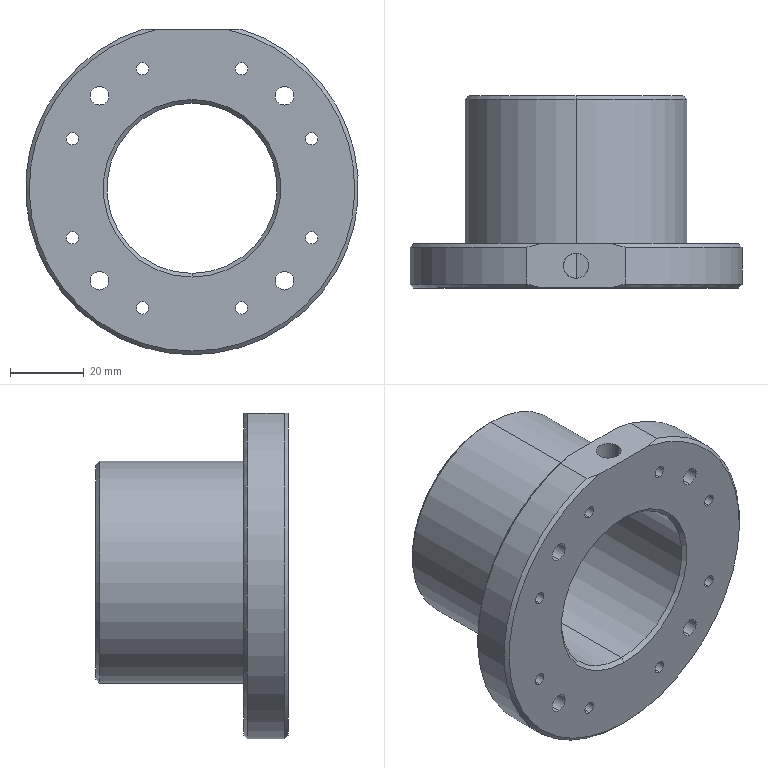Part | SolidWorks | features HoleWzd 3, ICE 3, Chamfer 1, CirPattern 1, Extrusion 1 | 1 solid | 45 faces | box 90 x 52 x 88 mm | volume 99604 mm3 | cylinder 32 | cone 9 | plane 4 | commonest cylinder face diameters 3.3 x16 5 x8 6.8 x2 46 x2 60 x2 90 x2